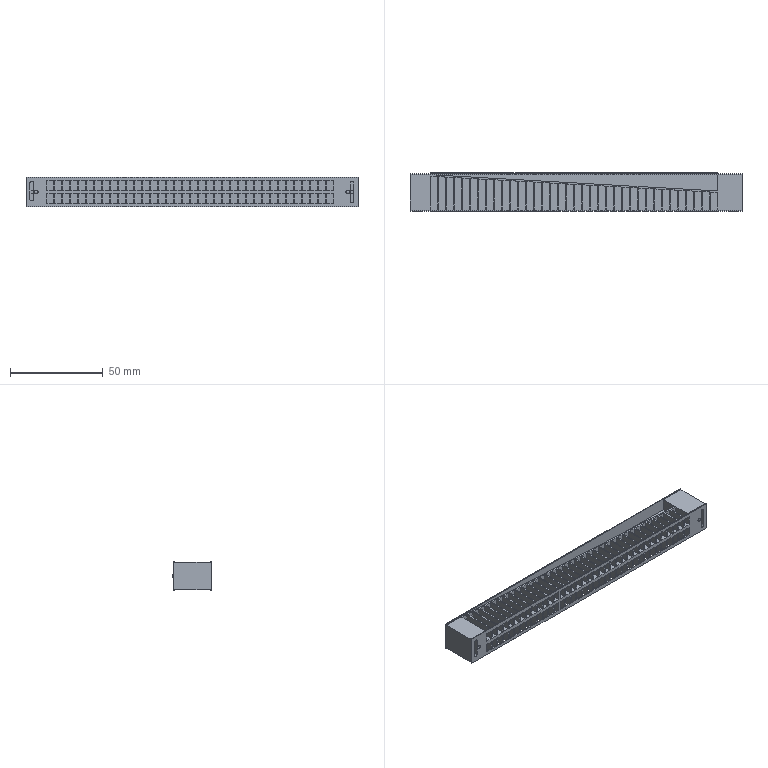Part | SolidWorks | features ICE 15, Extrusion 1, MirrorPattern 1 | 1 solid | 423 faces | box 178.568 x 20.5 x 16 mm | volume 18099 mm3 | plane 407 | cylinder 16 | commonest cylinder face diameters 2 x16